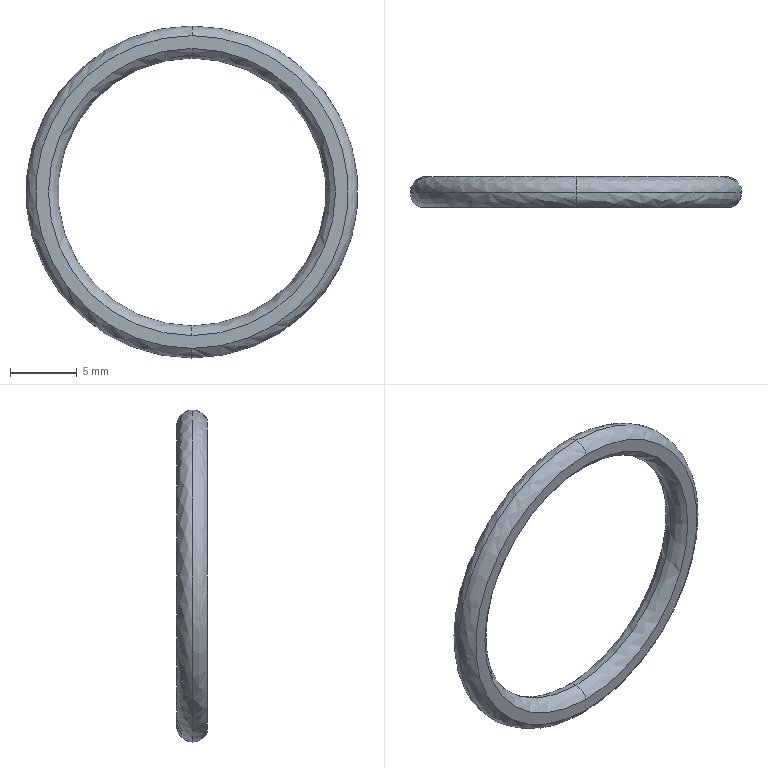Part | STEP file | PN_0034_default | 1 solid | 7 faces | box 24.8 x 2.3 x 24.8 mm | volume 313.815 mm3 | spline 6 | plane 1
STEP:
#1=CARTESIAN_POINT('',(0.,0.,0.));
#2=DIRECTION('',(0.,0.,1.));
#3=DIRECTION('',(1.,0.,0.));
#4=AXIS2_PLACEMENT_3D('',#1,#2,#3);
#5=CARTESIAN_POINT('',(0.,0.,10.));
#6=VERTEX_POINT('',#5);
#7=CARTESIAN_POINT('',(0.,0.,-10.));
#8=VERTEX_POINT('',#7);
#9=CARTESIAN_POINT('',(0.,0.,0.));
#10=DIRECTION('',(0.,-1.,0.));
#11=DIRECTION('',(0.,0.,-1.));
#12=AXIS2_PLACEMENT_3D('',#9,#10,#11);
#13=CIRCLE('',#12,10.);
#14=CARTESIAN_POINT('',(0.,0.,10.));
#15=CARTESIAN_POINT('',(-20.,0.,10.));
#16=CARTESIAN_POINT('',(-20.,0.,-10.));
#17=CARTESIAN_POINT('',(0.,0.,-10.));
#18=CARTESIAN_POINT('',(0.,-0.4919,10.));
#19=CARTESIAN_POINT('',(-20.,-0.4919,10.));
#20=CARTESIAN_POINT('',(-20.,-0.4919,-10.));
#21=CARTESIAN_POINT('',(0.,-0.4919,-10.));
#22=CARTESIAN_POINT('',(0.,-0.9034,10.27));
#23=CARTESIAN_POINT('',(-20.539,-0.9034,10.27));
#24=CARTESIAN_POINT('',(-20.539,-0.9034,-10.27));
#25=CARTESIAN_POINT('',(0.,-0.9034,-10.27));
#26=CARTESIAN_POINT('',(0.,-1.1,10.72));
#27=CARTESIAN_POINT('',(-21.441,-1.1,10.72));
#28=CARTESIAN_POINT('',(-21.441,-1.1,-10.72));
#29=CARTESIAN_POINT('',(0.,-1.1,-10.72));
#30=(BOUNDED_SURFACE()B_SPLINE_SURFACE(3,3,((#14,#15,#16,#17),(#18,#19,#20,#21),(#22,#23,#24,#25),(#26,#27,#28,#29)),.UNSPECIFIED.,.F.,.F.,.F.)B_SPLINE_SURFACE_WITH_KNOTS((4,4),(4,4),(0.,1.),(0.,1.),.PIECEWISE_BEZIER_KNOTS.)GEOMETRIC_REPRESENTATION_ITEM()RATIONAL_B_SPLINE_SURFACE(((1.,0.3333,0.3333,1.),(0.891,0.297,0.297,0.891),(0.891,0.297,0.297,0.891),(1.,0.3333,0.3333,1.)))REPRESENTATION_ITEM('')SURFACE());
#31=CARTESIAN_POINT('',(0.,0.));
#32=CARTESIAN_POINT('',(0.,0.02375));
#33=CARTESIAN_POINT('',(0.,0.06805));
#34=CARTESIAN_POINT('',(0.,0.1267));
#35=CARTESIAN_POINT('',(0.,0.1794));
#36=CARTESIAN_POINT('',(0.,0.2276));
#37=CARTESIAN_POINT('',(0.,0.2721));
#38=CARTESIAN_POINT('',(0.,0.3139));
#39=CARTESIAN_POINT('',(0.,0.3535));
#40=CARTESIAN_POINT('',(0.,0.3914));
#41=CARTESIAN_POINT('',(0.,0.4282));
#42=CARTESIAN_POINT('',(0.,0.4643));
#43=CARTESIAN_POINT('',(0.,0.5));
#44=CARTESIAN_POINT('',(0.,0.5357));
#45=CARTESIAN_POINT('',(0.,0.5718));
#46=CARTESIAN_POINT('',(0.,0.6086));
#47=CARTESIAN_POINT('',(0.,0.6465));
#48=CARTESIAN_POINT('',(0.,0.6861));
#49=CARTESIAN_POINT('',(0.,0.7279));
#50=CARTESIAN_POINT('',(0.,0.7724));
#51=CARTESIAN_POINT('',(0.,0.8206));
#52=CARTESIAN_POINT('',(0.,0.8733));
#53=CARTESIAN_POINT('',(0.,0.9319));
#54=CARTESIAN_POINT('',(0.,0.9763));
#55=CARTESIAN_POINT('',(0.,1.));
#56=B_SPLINE_CURVE_WITH_KNOTS('',3,(#31,#32,#33,#34,#35,#36,#37,#38,#39,#40,#41,#42,#43,#44,#45,#46,#47,#48,#49,#50,#51,#52,#53,#54,#55),.UNSPECIFIED.,.F.,.F.,(4,1,1,1,1,1,1,1,1,1,1,1,1,1,1,1,1,1,1,1,1,1,4),(3.142,3.284,3.427,3.57,3.713,3.856,3.998,4.141,4.284,4.427,4.57,4.712,4.855,4.998,5.141,5.284,5.426,5.569,5.712,5.855,5.998,6.14,6.283),.QUASI_UNIFORM_KNOTS.);
#57=(GEOMETRIC_REPRESENTATION_CONTEXT(2)PARAMETRIC_REPRESENTATION_CONTEXT()REPRESENTATION_CONTEXT('',''));
#58=DEFINITIONAL_REPRESENTATION('',(#56),#57);
#59=PCURVE('',#30,#58);
#60=CARTESIAN_POINT('',(0.,0.,12.4));
#61=CARTESIAN_POINT('',(-24.8,0.,12.4));
#62=CARTESIAN_POINT('',(-24.8,0.,-12.4));
#63=CARTESIAN_POINT('',(0.,0.,-12.4));
#64=CARTESIAN_POINT('',(0.,2.4,12.4));
#65=CARTESIAN_POINT('',(-24.8,2.4,12.4));
#66=CARTESIAN_POINT('',(-24.8,2.4,-12.4));
#67=CARTESIAN_POINT('',(0.,2.4,-12.4));
#68=CARTESIAN_POINT('',(0.,2.4,10.));
#69=CARTESIAN_POINT('',(-20.,2.4,10.));
#70=CARTESIAN_POINT('',(-20.,2.4,-10.));
#71=CARTESIAN_POINT('',(0.,2.4,-10.));
#72=CARTESIAN_POINT('',(0.,0.,10.));
#73=CARTESIAN_POINT('',(-20.,0.,10.));
#74=CARTESIAN_POINT('',(-20.,0.,-10.));
#75=CARTESIAN_POINT('',(0.,0.,-10.));
#76=(BOUNDED_SURFACE()B_SPLINE_SURFACE(3,3,((#60,#61,#62,#63),(#64,#65,#66,#67),(#68,#69,#70,#71),(#72,#73,#74,#75)),.UNSPECIFIED.,.F.,.F.,.F.)B_SPLINE_SURFACE_WITH_KNOTS((4,4),(4,4),(0.,1.),(0.,1.),.PIECEWISE_BEZIER_KNOTS.)GEOMETRIC_REPRESENTATION_ITEM()RATIONAL_B_SPLINE_SURFACE(((1.,0.3333,0.3333,1.),(0.3333,0.1111,0.1111,0.3333),(0.3333,0.1111,0.1111,0.3333),(1.,0.3333,0.3333,1.)))REPRESENTATION_ITEM('')SURFACE());
#77=CARTESIAN_POINT('',(1.,0.));
#78=CARTESIAN_POINT('',(1.,0.02375));
#79=CARTESIAN_POINT('',(1.,0.06805));
#80=CARTESIAN_POINT('',(1.,0.1267));
#81=CARTESIAN_POINT('',(1.,0.1794));
#82=CARTESIAN_POINT('',(1.,0.2276));
#83=CARTESIAN_POINT('',(1.,0.2721));
#84=CARTESIAN_POINT('',(1.,0.3139));
#85=CARTESIAN_POINT('',(1.,0.3535));
#86=CARTESIAN_POINT('',(1.,0.3914));
#87=CARTESIAN_POINT('',(1.,0.4282));
#88=CARTESIAN_POINT('',(1.,0.4643));
#89=CARTESIAN_POINT('',(1.,0.5));
#90=CARTESIAN_POINT('',(1.,0.5357));
#91=CARTESIAN_POINT('',(1.,0.5718));
#92=CARTESIAN_POINT('',(1.,0.6086));
#93=CARTESIAN_POINT('',(1.,0.6465));
#94=CARTESIAN_POINT('',(1.,0.6861));
#95=CARTESIAN_POINT('',(1.,0.7279));
#96=CARTESIAN_POINT('',(1.,0.7724));
#97=CARTESIAN_POINT('',(1.,0.8206));
#98=CARTESIAN_POINT('',(1.,0.8733));
#99=CARTESIAN_POINT('',(1.,0.9319));
#100=CARTESIAN_POINT('',(1.,0.9763));
#101=CARTESIAN_POINT('',(1.,1.));
#102=B_SPLINE_CURVE_WITH_KNOTS('',3,(#77,#78,#79,#80,#81,#82,#83,#84,#85,#86,#87,#88,#89,#90,#91,#92,#93,#94,#95,#96,#97,#98,#99,#100,#101),.UNSPECIFIED.,.F.,.F.,(4,1,1,1,1,1,1,1,1,1,1,1,1,1,1,1,1,1,1,1,1,1,4),(3.142,3.284,3.427,3.57,3.713,3.856,3.998,4.141,4.284,4.427,4.57,4.712,4.855,4.998,5.141,5.284,5.426,5.569,5.712,5.855,5.998,6.14,6.283),.QUASI_UNIFORM_KNOTS.);
#103=(GEOMETRIC_REPRESENTATION_CONTEXT(2)PARAMETRIC_REPRESENTATION_CONTEXT()REPRESENTATION_CONTEXT('',''));
#104=DEFINITIONAL_REPRESENTATION('',(#102),#103);
#105=PCURVE('',#76,#104);
#106=SURFACE_CURVE('',#13,(#59,#105),.PCURVE_S1.);
#107=EDGE_CURVE('',#6,#8,#106,.T.);
#108=ORIENTED_EDGE('',*,*,#107,.F.);
#109=CARTESIAN_POINT('',(0.,-1.1,10.72));
#110=VERTEX_POINT('',#109);
#111=CARTESIAN_POINT('',(0.,0.,11.2));
#112=DIRECTION('',(-1.,0.,0.));
#113=DIRECTION('',(0.,0.,1.));
#114=AXIS2_PLACEMENT_3D('',#111,#112,#113);
#115=CIRCLE('',#114,1.2);
#116=CARTESIAN_POINT('',(0.,0.));
#117=CARTESIAN_POINT('',(0.01603,0.));
#118=CARTESIAN_POINT('',(0.04785,0.));
#119=CARTESIAN_POINT('',(0.09491,0.));
#120=CARTESIAN_POINT('',(0.1414,0.));
#121=CARTESIAN_POINT('',(0.1873,0.));
#122=CARTESIAN_POINT('',(0.2328,0.));
#123=CARTESIAN_POINT('',(0.2779,0.));
#124=CARTESIAN_POINT('',(0.3227,0.));
#125=CARTESIAN_POINT('',(0.3672,0.));
#126=CARTESIAN_POINT('',(0.4116,0.));
#127=CARTESIAN_POINT('',(0.4558,0.));
#128=CARTESIAN_POINT('',(0.5,0.));
#129=CARTESIAN_POINT('',(0.5442,0.));
#130=CARTESIAN_POINT('',(0.5884,0.));
#131=CARTESIAN_POINT('',(0.6328,0.));
#132=CARTESIAN_POINT('',(0.6773,0.));
#133=CARTESIAN_POINT('',(0.7221,0.));
#134=CARTESIAN_POINT('',(0.7672,0.));
#135=CARTESIAN_POINT('',(0.8127,0.));
#136=CARTESIAN_POINT('',(0.8586,0.));
#137=CARTESIAN_POINT('',(0.9051,0.));
#138=CARTESIAN_POINT('',(0.9521,0.));
#139=CARTESIAN_POINT('',(0.984,0.));
#140=CARTESIAN_POINT('',(1.,0.));
#141=B_SPLINE_CURVE_WITH_KNOTS('',3,(#116,#117,#118,#119,#120,#121,#122,#123,#124,#125,#126,#127,#128,#129,#130,#131,#132,#133,#134,#135,#136,#137,#138,#139,#140),.UNSPECIFIED.,.F.,.F.,(4,1,1,1,1,1,1,1,1,1,1,1,1,1,1,1,1,1,1,1,1,1,4),(3.142,3.194,3.247,3.3,3.352,3.405,3.458,3.511,3.563,3.616,3.669,3.721,3.774,3.827,3.88,3.932,3.985,4.038,4.09,4.143,4.196,4.249,4.301),.QUASI_UNIFORM_KNOTS.);
#142=(GEOMETRIC_REPRESENTATION_CONTEXT(2)PARAMETRIC_REPRESENTATION_CONTEXT()REPRESENTATION_CONTEXT('',''));
#143=DEFINITIONAL_REPRESENTATION('',(#141),#142);
#144=PCURVE('',#30,#143);
#145=CARTESIAN_POINT('',(0.,0.,-10.));
#146=CARTESIAN_POINT('',(20.,0.,-10.));
#147=CARTESIAN_POINT('',(20.,0.,10.));
#148=CARTESIAN_POINT('',(0.,0.,10.));
#149=CARTESIAN_POINT('',(0.,-0.4919,-10.));
#150=CARTESIAN_POINT('',(20.,-0.4919,-10.));
#151=CARTESIAN_POINT('',(20.,-0.4919,10.));
#152=CARTESIAN_POINT('',(0.,-0.4919,10.));
#153=CARTESIAN_POINT('',(0.,-0.9034,-10.27));
#154=CARTESIAN_POINT('',(20.539,-0.9034,-10.27));
#155=CARTESIAN_POINT('',(20.539,-0.9034,10.27));
#156=CARTESIAN_POINT('',(0.,-0.9034,10.27));
#157=CARTESIAN_POINT('',(0.,-1.1,-10.72));
#158=CARTESIAN_POINT('',(21.441,-1.1,-10.72));
#159=CARTESIAN_POINT('',(21.441,-1.1,10.72));
#160=CARTESIAN_POINT('',(0.,-1.1,10.72));
#161=(BOUNDED_SURFACE()B_SPLINE_SURFACE(3,3,((#145,#146,#147,#148),(#149,#150,#151,#152),(#153,#154,#155,#156),(#157,#158,#159,#160)),.UNSPECIFIED.,.F.,.F.,.F.)B_SPLINE_SURFACE_WITH_KNOTS((4,4),(4,4),(0.,1.),(0.,1.),.PIECEWISE_BEZIER_KNOTS.)GEOMETRIC_REPRESENTATION_ITEM()RATIONAL_B_SPLINE_SURFACE(((1.,0.3333,0.3333,1.),(0.891,0.297,0.297,0.891),(0.891,0.297,0.297,0.891),(1.,0.3333,0.3333,1.)))REPRESENTATION_ITEM('')SURFACE());
#162=CARTESIAN_POINT('',(0.,1.));
#163=CARTESIAN_POINT('',(0.01603,1.));
#164=CARTESIAN_POINT('',(0.04785,1.));
#165=CARTESIAN_POINT('',(0.09491,1.));
#166=CARTESIAN_POINT('',(0.1414,1.));
#167=CARTESIAN_POINT('',(0.1873,1.));
#168=CARTESIAN_POINT('',(0.2328,1.));
#169=CARTESIAN_POINT('',(0.2779,1.));
#170=CARTESIAN_POINT('',(0.3227,1.));
#171=CARTESIAN_POINT('',(0.3672,1.));
#172=CARTESIAN_POINT('',(0.4116,1.));
#173=CARTESIAN_POINT('',(0.4558,1.));
#174=CARTESIAN_POINT('',(0.5,1.));
#175=CARTESIAN_POINT('',(0.5442,1.));
#176=CARTESIAN_POINT('',(0.5884,1.));
#177=CARTESIAN_POINT('',(0.6328,1.));
#178=CARTESIAN_POINT('',(0.6773,1.));
#179=CARTESIAN_POINT('',(0.7221,1.));
#180=CARTESIAN_POINT('',(0.7672,1.));
#181=CARTESIAN_POINT('',(0.8127,1.));
#182=CARTESIAN_POINT('',(0.8586,1.));
#183=CARTESIAN_POINT('',(0.9051,1.));
#184=CARTESIAN_POINT('',(0.9521,1.));
#185=CARTESIAN_POINT('',(0.984,1.));
#186=CARTESIAN_POINT('',(1.,1.));
#187=B_SPLINE_CURVE_WITH_KNOTS('',3,(#162,#163,#164,#165,#166,#167,#168,#169,#170,#171,#172,#173,#174,#175,#176,#177,#178,#179,#180,#181,#182,#183,#184,#185,#186),.UNSPECIFIED.,.F.,.F.,(4,1,1,1,1,1,1,1,1,1,1,1,1,1,1,1,1,1,1,1,1,1,4),(3.142,3.194,3.247,3.3,3.352,3.405,3.458,3.511,3.563,3.616,3.669,3.721,3.774,3.827,3.88,3.932,3.985,4.038,4.09,4.143,4.196,4.249,4.301),.QUASI_UNIFORM_KNOTS.);
#188=(GEOMETRIC_REPRESENTATION_CONTEXT(2)PARAMETRIC_REPRESENTATION_CONTEXT()REPRESENTATION_CONTEXT('',''));
#189=DEFINITIONAL_REPRESENTATION('',(#187),#188);
#190=PCURVE('',#161,#189);
#191=SURFACE_CURVE('',#115,(#144,#190),.PCURVE_S1.);
#192=EDGE_CURVE('',#6,#110,#191,.T.);
#193=ORIENTED_EDGE('',*,*,#192,.T.);
#194=CARTESIAN_POINT('',(0.,-1.1,-10.72));
#195=VERTEX_POINT('',#194);
#196=CARTESIAN_POINT('',(0.,-1.1,0.));
#197=DIRECTION('',(0.,-1.,0.));
#198=DIRECTION('',(0.,0.,-1.));
#199=AXIS2_PLACEMENT_3D('',#196,#197,#198);
#200=CIRCLE('',#199,10.72);
#201=CARTESIAN_POINT('',(1.,0.));
#202=CARTESIAN_POINT('',(1.,0.02375));
#203=CARTESIAN_POINT('',(1.,0.06805));
#204=CARTESIAN_POINT('',(1.,0.1267));
#205=CARTESIAN_POINT('',(1.,0.1794));
#206=CARTESIAN_POINT('',(1.,0.2276));
#207=CARTESIAN_POINT('',(1.,0.2721));
#208=CARTESIAN_POINT('',(1.,0.3139));
#209=CARTESIAN_POINT('',(1.,0.3535));
#210=CARTESIAN_POINT('',(1.,0.3914));
#211=CARTESIAN_POINT('',(1.,0.4282));
#212=CARTESIAN_POINT('',(1.,0.4643));
#213=CARTESIAN_POINT('',(1.,0.5));
#214=CARTESIAN_POINT('',(1.,0.5357));
#215=CARTESIAN_POINT('',(1.,0.5718));
#216=CARTESIAN_POINT('',(1.,0.6086));
#217=CARTESIAN_POINT('',(1.,0.6465));
#218=CARTESIAN_POINT('',(1.,0.6861));
#219=CARTESIAN_POINT('',(1.,0.7279));
#220=CARTESIAN_POINT('',(1.,0.7724));
#221=CARTESIAN_POINT('',(1.,0.8206));
#222=CARTESIAN_POINT('',(1.,0.8733));
#223=CARTESIAN_POINT('',(1.,0.9319));
#224=CARTESIAN_POINT('',(1.,0.9763));
#225=CARTESIAN_POINT('',(1.,1.));
#226=B_SPLINE_CURVE_WITH_KNOTS('',3,(#201,#202,#203,#204,#205,#206,#207,#208,#209,#210,#211,#212,#213,#214,#215,#216,#217,#218,#219,#220,#221,#222,#223,#224,#225),.UNSPECIFIED.,.F.,.F.,(4,1,1,1,1,1,1,1,1,1,1,1,1,1,1,1,1,1,1,1,1,1,4),(3.142,3.284,3.427,3.57,3.713,3.856,3.998,4.141,4.284,4.427,4.57,4.712,4.855,4.998,5.141,5.284,5.426,5.569,5.712,5.855,5.998,6.14,6.283),.QUASI_UNIFORM_KNOTS.);
#227=(GEOMETRIC_REPRESENTATION_CONTEXT(2)PARAMETRIC_REPRESENTATION_CONTEXT()REPRESENTATION_CONTEXT('',''));
#228=DEFINITIONAL_REPRESENTATION('',(#226),#227);
#229=PCURVE('',#30,#228);
#230=CARTESIAN_POINT('',(11.2,-1.1,0.));
#231=DIRECTION('',(0.,-1.,0.));
#232=DIRECTION('',(0.,0.,-1.));
#233=AXIS2_PLACEMENT_3D('',#230,#231,#232);
#234=PLANE('',#233);
#235=CARTESIAN_POINT('',(0.,-11.2));
#236=DIRECTION('',(1.,0.));
#237=AXIS2_PLACEMENT_2D('',#235,#236);
#238=CIRCLE('',#237,10.72);
#239=(GEOMETRIC_REPRESENTATION_CONTEXT(2)PARAMETRIC_REPRESENTATION_CONTEXT()REPRESENTATION_CONTEXT('',''));
#240=DEFINITIONAL_REPRESENTATION('',(#238),#239);
#241=PCURVE('',#234,#240);
#242=SURFACE_CURVE('',#200,(#229,#241),.PCURVE_S1.);
#243=EDGE_CURVE('',#110,#195,#242,.T.);
#244=ORIENTED_EDGE('',*,*,#243,.T.);
#245=CARTESIAN_POINT('',(0.,0.,-11.2));
#246=DIRECTION('',(1.,0.,0.));
#247=DIRECTION('',(0.,0.,-1.));
#248=AXIS2_PLACEMENT_3D('',#245,#246,#247);
#249=CIRCLE('',#248,1.2);
#250=CARTESIAN_POINT('',(0.,1.));
#251=CARTESIAN_POINT('',(0.01603,1.));
#252=CARTESIAN_POINT('',(0.04785,1.));
#253=CARTESIAN_POINT('',(0.09491,1.));
#254=CARTESIAN_POINT('',(0.1414,1.));
#255=CARTESIAN_POINT('',(0.1873,1.));
#256=CARTESIAN_POINT('',(0.2328,1.));
#257=CARTESIAN_POINT('',(0.2779,1.));
#258=CARTESIAN_POINT('',(0.3227,1.));
#259=CARTESIAN_POINT('',(0.3672,1.));
#260=CARTESIAN_POINT('',(0.4116,1.));
#261=CARTESIAN_POINT('',(0.4558,1.));
#262=CARTESIAN_POINT('',(0.5,1.));
#263=CARTESIAN_POINT('',(0.5442,1.));
#264=CARTESIAN_POINT('',(0.5884,1.));
#265=CARTESIAN_POINT('',(0.6328,1.));
#266=CARTESIAN_POINT('',(0.6773,1.));
#267=CARTESIAN_POINT('',(0.7221,1.));
#268=CARTESIAN_POINT('',(0.7672,1.));
#269=CARTESIAN_POINT('',(0.8127,1.));
#270=CARTESIAN_POINT('',(0.8586,1.));
#271=CARTESIAN_POINT('',(0.9051,1.));
#272=CARTESIAN_POINT('',(0.9521,1.));
#273=CARTESIAN_POINT('',(0.984,1.));
#274=CARTESIAN_POINT('',(1.,1.));
#275=B_SPLINE_CURVE_WITH_KNOTS('',3,(#250,#251,#252,#253,#254,#255,#256,#257,#258,#259,#260,#261,#262,#263,#264,#265,#266,#267,#268,#269,#270,#271,#272,#273,#274),.UNSPECIFIED.,.F.,.F.,(4,1,1,1,1,1,1,1,1,1,1,1,1,1,1,1,1,1,1,1,1,1,4),(3.142,3.194,3.247,3.3,3.352,3.405,3.458,3.511,3.563,3.616,3.669,3.721,3.774,3.827,3.88,3.932,3.985,4.038,4.09,4.143,4.196,4.249,4.301),.QUASI_UNIFORM_KNOTS.);
#276=(GEOMETRIC_REPRESENTATION_CONTEXT(2)PARAMETRIC_REPRESENTATION_CONTEXT()REPRESENTATION_CONTEXT('',''));
#277=DEFINITIONAL_REPRESENTATION('',(#275),#276);
#278=PCURVE('',#30,#277);
#279=CARTESIAN_POINT('',(0.,0.));
#280=CARTESIAN_POINT('',(0.01603,0.));
#281=CARTESIAN_POINT('',(0.04785,0.));
#282=CARTESIAN_POINT('',(0.09491,0.));
#283=CARTESIAN_POINT('',(0.1414,0.));
#284=CARTESIAN_POINT('',(0.1873,0.));
#285=CARTESIAN_POINT('',(0.2328,0.));
#286=CARTESIAN_POINT('',(0.2779,0.));
#287=CARTESIAN_POINT('',(0.3227,0.));
#288=CARTESIAN_POINT('',(0.3672,0.));
#289=CARTESIAN_POINT('',(0.4116,0.));
#290=CARTESIAN_POINT('',(0.4558,0.));
#291=CARTESIAN_POINT('',(0.5,0.));
#292=CARTESIAN_POINT('',(0.5442,0.));
#293=CARTESIAN_POINT('',(0.5884,0.));
#294=CARTESIAN_POINT('',(0.6328,0.));
#295=CARTESIAN_POINT('',(0.6773,0.));
#296=CARTESIAN_POINT('',(0.7221,0.));
#297=CARTESIAN_POINT('',(0.7672,0.));
#298=CARTESIAN_POINT('',(0.8127,0.));
#299=CARTESIAN_POINT('',(0.8586,0.));
#300=CARTESIAN_POINT('',(0.9051,0.));
#301=CARTESIAN_POINT('',(0.9521,0.));
#302=CARTESIAN_POINT('',(0.984,0.));
#303=CARTESIAN_POINT('',(1.,0.));
#304=B_SPLINE_CURVE_WITH_KNOTS('',3,(#279,#280,#281,#282,#283,#284,#285,#286,#287,#288,#289,#290,#291,#292,#293,#294,#295,#296,#297,#298,#299,#300,#301,#302,#303),.UNSPECIFIED.,.F.,.F.,(4,1,1,1,1,1,1,1,1,1,1,1,1,1,1,1,1,1,1,1,1,1,4),(3.142,3.194,3.247,3.3,3.352,3.405,3.458,3.511,3.563,3.616,3.669,3.721,3.774,3.827,3.88,3.932,3.985,4.038,4.09,4.143,4.196,4.249,4.301),.QUASI_UNIFORM_KNOTS.);
#305=(GEOMETRIC_REPRESENTATION_CONTEXT(2)PARAMETRIC_REPRESENTATION_CONTEXT()REPRESENTATION_CONTEXT('',''));
#306=DEFINITIONAL_REPRESENTATION('',(#304),#305);
#307=PCURVE('',#161,#306);
#308=SURFACE_CURVE('',#249,(#278,#307),.PCURVE_S1.);
#309=EDGE_CURVE('',#8,#195,#308,.T.);
#310=ORIENTED_EDGE('',*,*,#309,.F.);
#311=EDGE_LOOP('',(#108,#193,#244,#310));
#312=FACE_BOUND('',#311,.T.);
#313=ADVANCED_FACE('',(#312),#30,.T.);
#314=CARTESIAN_POINT('',(0.,-1.1,-11.68));
#315=VERTEX_POINT('',#314);
#316=CARTESIAN_POINT('',(0.,-1.1,11.68));
#317=VERTEX_POINT('',#316);
#318=CARTESIAN_POINT('',(0.,-1.1,0.));
#319=DIRECTION('',(0.,1.,0.));
#320=DIRECTION('',(0.,0.,-1.));
#321=AXIS2_PLACEMENT_3D('',#318,#319,#320);
#322=CIRCLE('',#321,11.68);
#323=CARTESIAN_POINT('',(0.,-1.1,11.68));
#324=CARTESIAN_POINT('',(-23.359,-1.1,11.68));
#325=CARTESIAN_POINT('',(-23.359,-1.1,-11.68));
#326=CARTESIAN_POINT('',(0.,-1.1,-11.68));
#327=CARTESIAN_POINT('',(0.,-0.9034,12.13));
#328=CARTESIAN_POINT('',(-24.261,-0.9034,12.13));
#329=CARTESIAN_POINT('',(-24.261,-0.9034,-12.13));
#330=CARTESIAN_POINT('',(0.,-0.9034,-12.13));
#331=CARTESIAN_POINT('',(0.,-0.4919,12.4));
#332=CARTESIAN_POINT('',(-24.8,-0.4919,12.4));
#333=CARTESIAN_POINT('',(-24.8,-0.4919,-12.4));
#334=CARTESIAN_POINT('',(0.,-0.4919,-12.4));
#335=CARTESIAN_POINT('',(0.,0.,12.4));
#336=CARTESIAN_POINT('',(-24.8,0.,12.4));
#337=CARTESIAN_POINT('',(-24.8,0.,-12.4));
#338=CARTESIAN_POINT('',(0.,0.,-12.4));
#339=(BOUNDED_SURFACE()B_SPLINE_SURFACE(3,3,((#323,#324,#325,#326),(#327,#328,#329,#330),(#331,#332,#333,#334),(#335,#336,#337,#338)),.UNSPECIFIED.,.F.,.F.,.F.)B_SPLINE_SURFACE_WITH_KNOTS((4,4),(4,4),(0.,1.),(0.,1.),.PIECEWISE_BEZIER_KNOTS.)GEOMETRIC_REPRESENTATION_ITEM()RATIONAL_B_SPLINE_SURFACE(((1.,0.3333,0.3333,1.),(0.891,0.297,0.297,0.891),(0.891,0.297,0.297,0.891),(1.,0.3333,0.3333,1.)))REPRESENTATION_ITEM('')SURFACE());
#340=CARTESIAN_POINT('',(0.,1.));
#341=CARTESIAN_POINT('',(0.,0.9763));
#342=CARTESIAN_POINT('',(0.,0.9319));
#343=CARTESIAN_POINT('',(0.,0.8733));
#344=CARTESIAN_POINT('',(0.,0.8206));
#345=CARTESIAN_POINT('',(0.,0.7724));
#346=CARTESIAN_POINT('',(0.,0.7279));
#347=CARTESIAN_POINT('',(0.,0.6861));
#348=CARTESIAN_POINT('',(0.,0.6465));
#349=CARTESIAN_POINT('',(0.,0.6086));
#350=CARTESIAN_POINT('',(0.,0.5718));
#351=CARTESIAN_POINT('',(0.,0.5357));
#352=CARTESIAN_POINT('',(0.,0.5));
#353=CARTESIAN_POINT('',(0.,0.4643));
#354=CARTESIAN_POINT('',(0.,0.4282));
#355=CARTESIAN_POINT('',(0.,0.3914));
#356=CARTESIAN_POINT('',(0.,0.3535));
#357=CARTESIAN_POINT('',(0.,0.3139));
#358=CARTESIAN_POINT('',(0.,0.2721));
#359=CARTESIAN_POINT('',(0.,0.2276));
#360=CARTESIAN_POINT('',(0.,0.1794));
#361=CARTESIAN_POINT('',(0.,0.1267));
#362=CARTESIAN_POINT('',(0.,0.06805));
#363=CARTESIAN_POINT('',(0.,0.02375));
#364=CARTESIAN_POINT('',(0.,0.));
#365=B_SPLINE_CURVE_WITH_KNOTS('',3,(#340,#341,#342,#343,#344,#345,#346,#347,#348,#349,#350,#351,#352,#353,#354,#355,#356,#357,#358,#359,#360,#361,#362,#363,#364),.UNSPECIFIED.,.F.,.F.,(4,1,1,1,1,1,1,1,1,1,1,1,1,1,1,1,1,1,1,1,1,1,4),(0.,0.1428,0.2856,0.4284,0.5712,0.714,0.8568,0.9996,1.142,1.285,1.428,1.571,1.714,1.856,1.999,2.142,2.285,2.428,2.57,2.713,2.856,2.999,3.142),.QUASI_UNIFORM_KNOTS.);
#366=(GEOMETRIC_REPRESENTATION_CONTEXT(2)PARAMETRIC_REPRESENTATION_CONTEXT()REPRESENTATION_CONTEXT('',''));
#367=DEFINITIONAL_REPRESENTATION('',(#365),#366);
#368=PCURVE('',#339,#367);
#369=CARTESIAN_POINT('',(11.68,-11.2));
#370=CARTESIAN_POINT('',(11.68,-31.43));
#371=CARTESIAN_POINT('',(-5.84,-21.315));
#372=CARTESIAN_POINT('',(-23.359,-11.2));
#373=CARTESIAN_POINT('',(-5.84,-1.085));
#374=CARTESIAN_POINT('',(11.68,9.03));
#375=CARTESIAN_POINT('',(11.68,-11.2));
#376=(BOUNDED_CURVE()B_SPLINE_CURVE(2,(#369,#370,#371,#372,#373,#374,#375),.UNSPECIFIED.,.T.,.F.)B_SPLINE_CURVE_WITH_KNOTS((1,2,2,2,2,1),(-2.094,0.,2.094,4.189,6.283,8.378),.UNSPECIFIED.)CURVE()GEOMETRIC_REPRESENTATION_ITEM()RATIONAL_B_SPLINE_CURVE((1.,0.5,1.,0.5,1.,0.5,1.))REPRESENTATION_ITEM(''));
#377=(GEOMETRIC_REPRESENTATION_CONTEXT(2)PARAMETRIC_REPRESENTATION_CONTEXT()REPRESENTATION_CONTEXT('',''));
#378=DEFINITIONAL_REPRESENTATION('',(#376),#377);
#379=PCURVE('',#234,#378);
#380=SURFACE_CURVE('',#322,(#368,#379),.PCURVE_S1.);
#381=EDGE_CURVE('',#315,#317,#380,.T.);
#382=ORIENTED_EDGE('',*,*,#381,.T.);
#383=CARTESIAN_POINT('',(0.,0.,12.4));
#384=VERTEX_POINT('',#383);
#385=CARTESIAN_POINT('',(0.,0.,11.2));
#386=DIRECTION('',(-1.,0.,0.));
#387=DIRECTION('',(0.,0.,1.));
#388=AXIS2_PLACEMENT_3D('',#385,#386,#387);
#389=CIRCLE('',#388,1.2);
#390=CARTESIAN_POINT('',(0.,0.));
#391=CARTESIAN_POINT('',(0.01603,0.));
#392=CARTESIAN_POINT('',(0.04785,0.));
#393=CARTESIAN_POINT('',(0.09491,0.));
#394=CARTESIAN_POINT('',(0.1414,0.));
#395=CARTESIAN_POINT('',(0.1873,0.));
#396=CARTESIAN_POINT('',(0.2328,0.));
#397=CARTESIAN_POINT('',(0.2779,0.));
#398=CARTESIAN_POINT('',(0.3227,0.));
#399=CARTESIAN_POINT('',(0.3672,0.));
#400=CARTESIAN_POINT('',(0.4116,0.));
#401=CARTESIAN_POINT('',(0.4558,0.));
#402=CARTESIAN_POINT('',(0.5,0.));
#403=CARTESIAN_POINT('',(0.5442,0.));
#404=CARTESIAN_POINT('',(0.5884,0.));
#405=CARTESIAN_POINT('',(0.6328,0.));
#406=CARTESIAN_POINT('',(0.6773,0.));
#407=CARTESIAN_POINT('',(0.7221,0.));
#408=CARTESIAN_POINT('',(0.7672,0.));
#409=CARTESIAN_POINT('',(0.8127,0.));
#410=CARTESIAN_POINT('',(0.8586,0.));
#411=CARTESIAN_POINT('',(0.9051,0.));
#412=CARTESIAN_POINT('',(0.9521,0.));
#413=CARTESIAN_POINT('',(0.984,0.));
#414=CARTESIAN_POINT('',(1.,0.));
#415=B_SPLINE_CURVE_WITH_KNOTS('',3,(#390,#391,#392,#393,#394,#395,#396,#397,#398,#399,#400,#401,#402,#403,#404,#405,#406,#407,#408,#409,#410,#411,#412,#413,#414),.UNSPECIFIED.,.F.,.F.,(4,1,1,1,1,1,1,1,1,1,1,1,1,1,1,1,1,1,1,1,1,1,4),(5.124,5.176,5.229,5.282,5.334,5.387,5.44,5.493,5.545,5.598,5.651,5.703,5.756,5.809,5.861,5.914,5.967,6.02,6.072,6.125,6.178,6.23,6.283),.QUASI_UNIFORM_KNOTS.);
#416=(GEOMETRIC_REPRESENTATION_CONTEXT(2)PARAMETRIC_REPRESENTATION_CONTEXT()REPRESENTATION_CONTEXT('',''));
#417=DEFINITIONAL_REPRESENTATION('',(#415),#416);
#418=PCURVE('',#339,#417);
#419=CARTESIAN_POINT('',(0.,-1.1,-11.68));
#420=CARTESIAN_POINT('',(23.359,-1.1,-11.68));
#421=CARTESIAN_POINT('',(23.359,-1.1,11.68));
#422=CARTESIAN_POINT('',(0.,-1.1,11.68));
#423=CARTESIAN_POINT('',(0.,-0.9034,-12.13));
#424=CARTESIAN_POINT('',(24.261,-0.9034,-12.13));
#425=CARTESIAN_POINT('',(24.261,-0.9034,12.13));
#426=CARTESIAN_POINT('',(0.,-0.9034,12.13));
#427=CARTESIAN_POINT('',(0.,-0.4919,-12.4));
#428=CARTESIAN_POINT('',(24.8,-0.4919,-12.4));
#429=CARTESIAN_POINT('',(24.8,-0.4919,12.4));
#430=CARTESIAN_POINT('',(0.,-0.4919,12.4));
#431=CARTESIAN_POINT('',(0.,0.,-12.4));
#432=CARTESIAN_POINT('',(24.8,0.,-12.4));
#433=CARTESIAN_POINT('',(24.8,0.,12.4));
#434=CARTESIAN_POINT('',(0.,0.,12.4));
#435=(BOUNDED_SURFACE()B_SPLINE_SURFACE(3,3,((#419,#420,#421,#422),(#423,#424,#425,#426),(#427,#428,#429,#430),(#431,#432,#433,#434)),.UNSPECIFIED.,.F.,.F.,.F.)B_SPLINE_SURFACE_WITH_KNOTS((4,4),(4,4),(0.,1.),(0.,1.),.PIECEWISE_BEZIER_KNOTS.)GEOMETRIC_REPRESENTATION_ITEM()RATIONAL_B_SPLINE_SURFACE(((1.,0.3333,0.3333,1.),(0.891,0.297,0.297,0.891),(0.891,0.297,0.297,0.891),(1.,0.3333,0.3333,1.)))REPRESENTATION_ITEM('')SURFACE());
#436=CARTESIAN_POINT('',(0.,1.));
#437=CARTESIAN_POINT('',(0.01603,1.));
#438=CARTESIAN_POINT('',(0.04785,1.));
#439=CARTESIAN_POINT('',(0.09491,1.));
#440=CARTESIAN_POINT('',(0.1414,1.));
#441=CARTESIAN_POINT('',(0.1873,1.));
#442=CARTESIAN_POINT('',(0.2328,1.));
#443=CARTESIAN_POINT('',(0.2779,1.));
#444=CARTESIAN_POINT('',(0.3227,1.));
#445=CARTESIAN_POINT('',(0.3672,1.));
#446=CARTESIAN_POINT('',(0.4116,1.));
#447=CARTESIAN_POINT('',(0.4558,1.));
#448=CARTESIAN_POINT('',(0.5,1.));
#449=CARTESIAN_POINT('',(0.5442,1.));
#450=CARTESIAN_POINT('',(0.5884,1.));
#451=CARTESIAN_POINT('',(0.6328,1.));
#452=CARTESIAN_POINT('',(0.6773,1.));
#453=CARTESIAN_POINT('',(0.7221,1.));
#454=CARTESIAN_POINT('',(0.7672,1.));
#455=CARTESIAN_POINT('',(0.8127,1.));
#456=CARTESIAN_POINT('',(0.8586,1.));
#457=CARTESIAN_POINT('',(0.9051,1.));
#458=CARTESIAN_POINT('',(0.9521,1.));
#459=CARTESIAN_POINT('',(0.984,1.));
#460=CARTESIAN_POINT('',(1.,1.));
#461=B_SPLINE_CURVE_WITH_KNOTS('',3,(#436,#437,#438,#439,#440,#441,#442,#443,#444,#445,#446,#447,#448,#449,#450,#451,#452,#453,#454,#455,#456,#457,#458,#459,#460),.UNSPECIFIED.,.F.,.F.,(4,1,1,1,1,1,1,1,1,1,1,1,1,1,1,1,1,1,1,1,1,1,4),(5.124,5.176,5.229,5.282,5.334,5.387,5.44,5.493,5.545,5.598,5.651,5.703,5.756,5.809,5.861,5.914,5.967,6.02,6.072,6.125,6.178,6.23,6.283),.QUASI_UNIFORM_KNOTS.);
#462=(GEOMETRIC_REPRESENTATION_CONTEXT(2)PARAMETRIC_REPRESENTATION_CONTEXT()REPRESENTATION_CONTEXT('',''));
#463=DEFINITIONAL_REPRESENTATION('',(#461),#462);
#464=PCURVE('',#435,#463);
#465=SURFACE_CURVE('',#389,(#418,#464),.PCURVE_S1.);
#466=EDGE_CURVE('',#317,#384,#465,.T.);
#467=ORIENTED_EDGE('',*,*,#466,.T.);
#468=CARTESIAN_POINT('',(0.,0.,-12.4));
#469=VERTEX_POINT('',#468);
#470=CARTESIAN_POINT('',(0.,0.,0.));
#471=DIRECTION('',(0.,-1.,0.));
#472=DIRECTION('',(0.,0.,-1.));
#473=AXIS2_PLACEMENT_3D('',#470,#471,#472);
#474=CIRCLE('',#473,12.4);
#475=CARTESIAN_POINT('',(1.,0.));
#476=CARTESIAN_POINT('',(1.,0.02375));
#477=CARTESIAN_POINT('',(1.,0.06805));
#478=CARTESIAN_POINT('',(1.,0.1267));
#479=CARTESIAN_POINT('',(1.,0.1794));
#480=CARTESIAN_POINT('',(1.,0.2276));
#481=CARTESIAN_POINT('',(1.,0.2721));
#482=CARTESIAN_POINT('',(1.,0.3139));
#483=CARTESIAN_POINT('',(1.,0.3535));
#484=CARTESIAN_POINT('',(1.,0.3914));
#485=CARTESIAN_POINT('',(1.,0.4282));
#486=CARTESIAN_POINT('',(1.,0.4643));
#487=CARTESIAN_POINT('',(1.,0.5));
#488=CARTESIAN_POINT('',(1.,0.5357));
#489=CARTESIAN_POINT('',(1.,0.5718));
#490=CARTESIAN_POINT('',(1.,0.6086));
#491=CARTESIAN_POINT('',(1.,0.6465));
#492=CARTESIAN_POINT('',(1.,0.6861));
#493=CARTESIAN_POINT('',(1.,0.7279));
#494=CARTESIAN_POINT('',(1.,0.7724));
#495=CARTESIAN_POINT('',(1.,0.8206));
#496=CARTESIAN_POINT('',(1.,0.8733));
#497=CARTESIAN_POINT('',(1.,0.9319));
#498=CARTESIAN_POINT('',(1.,0.9763));
#499=CARTESIAN_POINT('',(1.,1.));
#500=B_SPLINE_CURVE_WITH_KNOTS('',3,(#475,#476,#477,#478,#479,#480,#481,#482,#483,#484,#485,#486,#487,#488,#489,#490,#491,#492,#493,#494,#495,#496,#497,#498,#499),.UNSPECIFIED.,.F.,.F.,(4,1,1,1,1,1,1,1,1,1,1,1,1,1,1,1,1,1,1,1,1,1,4),(3.142,3.284,3.427,3.57,3.713,3.856,3.998,4.141,4.284,4.427,4.57,4.712,4.855,4.998,5.141,5.284,5.426,5.569,5.712,5.855,5.998,6.14,6.283),.QUASI_UNIFORM_KNOTS.);
#501=(GEOMETRIC_REPRESENTATION_CONTEXT(2)PARAMETRIC_REPRESENTATION_CONTEXT()REPRESENTATION_CONTEXT('',''));
#502=DEFINITIONAL_REPRESENTATION('',(#500),#501);
#503=PCURVE('',#339,#502);
#504=CARTESIAN_POINT('',(0.,0.));
#505=CARTESIAN_POINT('',(0.,0.02375));
#506=CARTESIAN_POINT('',(0.,0.06805));
#507=CARTESIAN_POINT('',(0.,0.1267));
#508=CARTESIAN_POINT('',(0.,0.1794));
#509=CARTESIAN_POINT('',(0.,0.2276));
#510=CARTESIAN_POINT('',(0.,0.2721));
#511=CARTESIAN_POINT('',(0.,0.3139));
#512=CARTESIAN_POINT('',(0.,0.3535));
#513=CARTESIAN_POINT('',(0.,0.3914));
#514=CARTESIAN_POINT('',(0.,0.4282));
#515=CARTESIAN_POINT('',(0.,0.4643));
#516=CARTESIAN_POINT('',(0.,0.5));
#517=CARTESIAN_POINT('',(0.,0.5357));
#518=CARTESIAN_POINT('',(0.,0.5718));
#519=CARTESIAN_POINT('',(0.,0.6086));
#520=CARTESIAN_POINT('',(0.,0.6465));
#521=CARTESIAN_POINT('',(0.,0.6861));
#522=CARTESIAN_POINT('',(0.,0.7279));
#523=CARTESIAN_POINT('',(0.,0.7724));
#524=CARTESIAN_POINT('',(0.,0.8206));
#525=CARTESIAN_POINT('',(0.,0.8733));
#526=CARTESIAN_POINT('',(0.,0.9319));
#527=CARTESIAN_POINT('',(0.,0.9763));
#528=CARTESIAN_POINT('',(0.,1.));
#529=B_SPLINE_CURVE_WITH_KNOTS('',3,(#504,#505,#506,#507,#508,#509,#510,#511,#512,#513,#514,#515,#516,#517,#518,#519,#520,#521,#522,#523,#524,#525,#526,#527,#528),.UNSPECIFIED.,.F.,.F.,(4,1,1,1,1,1,1,1,1,1,1,1,1,1,1,1,1,1,1,1,1,1,4),(3.142,3.284,3.427,3.57,3.713,3.856,3.998,4.141,4.284,4.427,4.57,4.712,4.855,4.998,5.141,5.284,5.426,5.569,5.712,5.855,5.998,6.14,6.283),.QUASI_UNIFORM_KNOTS.);
#530=(GEOMETRIC_REPRESENTATION_CONTEXT(2)PARAMETRIC_REPRESENTATION_CONTEXT()REPRESENTATION_CONTEXT('',''));
#531=DEFINITIONAL_REPRESENTATION('',(#529),#530);
#532=PCURVE('',#76,#531);
#533=SURFACE_CURVE('',#474,(#503,#532),.PCURVE_S1.);
#534=EDGE_CURVE('',#384,#469,#533,.T.);
#535=ORIENTED_EDGE('',*,*,#534,.T.);
#536=CARTESIAN_POINT('',(0.,0.,-11.2));
#537=DIRECTION('',(1.,0.,0.));
#538=DIRECTION('',(0.,0.,-1.));
#539=AXIS2_PLACEMENT_3D('',#536,#537,#538);
#540=CIRCLE('',#539,1.2);
#541=CARTESIAN_POINT('',(0.,1.));
#542=CARTESIAN_POINT('',(0.01603,1.));
#543=CARTESIAN_POINT('',(0.04785,1.));
#544=CARTESIAN_POINT('',(0.09491,1.));
#545=CARTESIAN_POINT('',(0.1414,1.));
#546=CARTESIAN_POINT('',(0.1873,1.));
#547=CARTESIAN_POINT('',(0.2328,1.));
#548=CARTESIAN_POINT('',(0.2779,1.));
#549=CARTESIAN_POINT('',(0.3227,1.));
#550=CARTESIAN_POINT('',(0.3672,1.));
#551=CARTESIAN_POINT('',(0.4116,1.));
#552=CARTESIAN_POINT('',(0.4558,1.));
#553=CARTESIAN_POINT('',(0.5,1.));
#554=CARTESIAN_POINT('',(0.5442,1.));
#555=CARTESIAN_POINT('',(0.5884,1.));
#556=CARTESIAN_POINT('',(0.6328,1.));
#557=CARTESIAN_POINT('',(0.6773,1.));
#558=CARTESIAN_POINT('',(0.7221,1.));
#559=CARTESIAN_POINT('',(0.7672,1.));
#560=CARTESIAN_POINT('',(0.8127,1.));
#561=CARTESIAN_POINT('',(0.8586,1.));
#562=CARTESIAN_POINT('',(0.9051,1.));
#563=CARTESIAN_POINT('',(0.9521,1.));
#564=CARTESIAN_POINT('',(0.984,1.));
#565=CARTESIAN_POINT('',(1.,1.));
#566=B_SPLINE_CURVE_WITH_KNOTS('',3,(#541,#542,#543,#544,#545,#546,#547,#548,#549,#550,#551,#552,#553,#554,#555,#556,#557,#558,#559,#560,#561,#562,#563,#564,#565),.UNSPECIFIED.,.F.,.F.,(4,1,1,1,1,1,1,1,1,1,1,1,1,1,1,1,1,1,1,1,1,1,4),(5.124,5.176,5.229,5.282,5.334,5.387,5.44,5.493,5.545,5.598,5.651,5.703,5.756,5.809,5.861,5.914,5.967,6.02,6.072,6.125,6.178,6.23,6.283),.QUASI_UNIFORM_KNOTS.);
#567=(GEOMETRIC_REPRESENTATION_CONTEXT(2)PARAMETRIC_REPRESENTATION_CONTEXT()REPRESENTATION_CONTEXT('',''));
#568=DEFINITIONAL_REPRESENTATION('',(#566),#567);
#569=PCURVE('',#339,#568);
#570=CARTESIAN_POINT('',(0.,0.));
#571=CARTESIAN_POINT('',(0.01603,0.));
#572=CARTESIAN_POINT('',(0.04785,0.));
#573=CARTESIAN_POINT('',(0.09491,0.));
#574=CARTESIAN_POINT('',(0.1414,0.));
#575=CARTESIAN_POINT('',(0.1873,0.));
#576=CARTESIAN_POINT('',(0.2328,0.));
#577=CARTESIAN_POINT('',(0.2779,0.));
#578=CARTESIAN_POINT('',(0.3227,0.));
#579=CARTESIAN_POINT('',(0.3672,0.));
#580=CARTESIAN_POINT('',(0.4116,0.));
#581=CARTESIAN_POINT('',(0.4558,0.));
#582=CARTESIAN_POINT('',(0.5,0.));
#583=CARTESIAN_POINT('',(0.5442,0.));
#584=CARTESIAN_POINT('',(0.5884,0.));
#585=CARTESIAN_POINT('',(0.6328,0.));
#586=CARTESIAN_POINT('',(0.6773,0.));
#587=CARTESIAN_POINT('',(0.7221,0.));
#588=CARTESIAN_POINT('',(0.7672,0.));
#589=CARTESIAN_POINT('',(0.8127,0.));
#590=CARTESIAN_POINT('',(0.8586,0.));
#591=CARTESIAN_POINT('',(0.9051,0.));
#592=CARTESIAN_POINT('',(0.9521,0.));
#593=CARTESIAN_POINT('',(0.984,0.));
#594=CARTESIAN_POINT('',(1.,0.));
#595=B_SPLINE_CURVE_WITH_KNOTS('',3,(#570,#571,#572,#573,#574,#575,#576,#577,#578,#579,#580,#581,#582,#583,#584,#585,#586,#587,#588,#589,#590,#591,#592,#593,#594),.UNSPECIFIED.,.F.,.F.,(4,1,1,1,1,1,1,1,1,1,1,1,1,1,1,1,1,1,1,1,1,1,4),(5.124,5.176,5.229,5.282,5.334,5.387,5.44,5.493,5.545,5.598,5.651,5.703,5.756,5.809,5.861,5.914,5.967,6.02,6.072,6.125,6.178,6.23,6.283),.QUASI_UNIFORM_KNOTS.);
#596=(GEOMETRIC_REPRESENTATION_CONTEXT(2)PARAMETRIC_REPRESENTATION_CONTEXT()REPRESENTATION_CONTEXT('',''));
#597=DEFINITIONAL_REPRESENTATION('',(#595),#596);
#598=PCURVE('',#435,#597);
#599=SURFACE_CURVE('',#540,(#569,#598),.PCURVE_S1.);
#600=EDGE_CURVE('',#315,#469,#599,.T.);
#601=ORIENTED_EDGE('',*,*,#600,.F.);
#602=EDGE_LOOP('',(#382,#467,#535,#601));
#603=FACE_BOUND('',#602,.T.);
#604=ADVANCED_FACE('',(#603),#339,.T.);
#605=ORIENTED_EDGE('',*,*,#534,.F.);
#606=CARTESIAN_POINT('',(0.,0.,11.2));
#607=DIRECTION('',(-1.,0.,0.));
#608=DIRECTION('',(0.,0.,1.));
#609=AXIS2_PLACEMENT_3D('',#606,#607,#608);
#610=CIRCLE('',#609,1.2);
#611=CARTESIAN_POINT('',(0.,0.));
#612=CARTESIAN_POINT('',(0.02375,0.));
#613=CARTESIAN_POINT('',(0.06805,0.));
#614=CARTESIAN_POINT('',(0.1267,0.));
#615=CARTESIAN_POINT('',(0.1794,0.));
#616=CARTESIAN_POINT('',(0.2276,0.));
#617=CARTESIAN_POINT('',(0.2721,0.));
#618=CARTESIAN_POINT('',(0.3139,0.));
#619=CARTESIAN_POINT('',(0.3535,0.));
#620=CARTESIAN_POINT('',(0.3914,0.));
#621=CARTESIAN_POINT('',(0.4282,0.));
#622=CARTESIAN_POINT('',(0.4643,0.));
#623=CARTESIAN_POINT('',(0.5,0.));
#624=CARTESIAN_POINT('',(0.5357,0.));
#625=CARTESIAN_POINT('',(0.5718,0.));
#626=CARTESIAN_POINT('',(0.6086,0.));
#627=CARTESIAN_POINT('',(0.6465,0.));
#628=CARTESIAN_POINT('',(0.6861,0.));
#629=CARTESIAN_POINT('',(0.7279,0.));
#630=CARTESIAN_POINT('',(0.7724,0.));
#631=CARTESIAN_POINT('',(0.8206,0.));
#632=CARTESIAN_POINT('',(0.8733,0.));
#633=CARTESIAN_POINT('',(0.9319,0.));
#634=CARTESIAN_POINT('',(0.9763,0.));
#635=CARTESIAN_POINT('',(1.,0.));
#636=B_SPLINE_CURVE_WITH_KNOTS('',3,(#611,#612,#613,#614,#615,#616,#617,#618,#619,#620,#621,#622,#623,#624,#625,#626,#627,#628,#629,#630,#631,#632,#633,#634,#635),.UNSPECIFIED.,.F.,.F.,(4,1,1,1,1,1,1,1,1,1,1,1,1,1,1,1,1,1,1,1,1,1,4),(0.,0.1428,0.2856,0.4284,0.5712,0.714,0.8568,0.9996,1.142,1.285,1.428,1.571,1.714,1.856,1.999,2.142,2.285,2.428,2.57,2.713,2.856,2.999,3.142),.QUASI_UNIFORM_KNOTS.);
#637=(GEOMETRIC_REPRESENTATION_CONTEXT(2)PARAMETRIC_REPRESENTATION_CONTEXT()REPRESENTATION_CONTEXT('',''));
#638=DEFINITIONAL_REPRESENTATION('',(#636),#637);
#639=PCURVE('',#76,#638);
#640=CARTESIAN_POINT('',(0.,0.,-12.4));
#641=CARTESIAN_POINT('',(24.8,0.,-12.4));
#642=CARTESIAN_POINT('',(24.8,0.,12.4));
#643=CARTESIAN_POINT('',(0.,0.,12.4));
#644=CARTESIAN_POINT('',(0.,2.4,-12.4));
#645=CARTESIAN_POINT('',(24.8,2.4,-12.4));
#646=CARTESIAN_POINT('',(24.8,2.4,12.4));
#647=CARTESIAN_POINT('',(0.,2.4,12.4));
#648=CARTESIAN_POINT('',(0.,2.4,-10.));
#649=CARTESIAN_POINT('',(20.,2.4,-10.));
#650=CARTESIAN_POINT('',(20.,2.4,10.));
#651=CARTESIAN_POINT('',(0.,2.4,10.));
#652=CARTESIAN_POINT('',(0.,0.,-10.));
#653=CARTESIAN_POINT('',(20.,0.,-10.));
#654=CARTESIAN_POINT('',(20.,0.,10.));
#655=CARTESIAN_POINT('',(0.,0.,10.));
#656=(BOUNDED_SURFACE()B_SPLINE_SURFACE(3,3,((#640,#641,#642,#643),(#644,#645,#646,#647),(#648,#649,#650,#651),(#652,#653,#654,#655)),.UNSPECIFIED.,.F.,.F.,.F.)B_SPLINE_SURFACE_WITH_KNOTS((4,4),(4,4),(0.,1.),(0.,1.),.PIECEWISE_BEZIER_KNOTS.)GEOMETRIC_REPRESENTATION_ITEM()RATIONAL_B_SPLINE_SURFACE(((1.,0.3333,0.3333,1.),(0.3333,0.1111,0.1111,0.3333),(0.3333,0.1111,0.1111,0.3333),(1.,0.3333,0.3333,1.)))REPRESENTATION_ITEM('')SURFACE());
#657=CARTESIAN_POINT('',(0.,1.));
#658=CARTESIAN_POINT('',(0.02375,1.));
#659=CARTESIAN_POINT('',(0.06805,1.));
#660=CARTESIAN_POINT('',(0.1267,1.));
#661=CARTESIAN_POINT('',(0.1794,1.));
#662=CARTESIAN_POINT('',(0.2276,1.));
#663=CARTESIAN_POINT('',(0.2721,1.));
#664=CARTESIAN_POINT('',(0.3139,1.));
#665=CARTESIAN_POINT('',(0.3535,1.));
#666=CARTESIAN_POINT('',(0.3914,1.));
#667=CARTESIAN_POINT('',(0.4282,1.));
#668=CARTESIAN_POINT('',(0.4643,1.));
#669=CARTESIAN_POINT('',(0.5,1.));
#670=CARTESIAN_POINT('',(0.5357,1.));
#671=CARTESIAN_POINT('',(0.5718,1.));
#672=CARTESIAN_POINT('',(0.6086,1.));
#673=CARTESIAN_POINT('',(0.6465,1.));
#674=CARTESIAN_POINT('',(0.6861,1.));
#675=CARTESIAN_POINT('',(0.7279,1.));
#676=CARTESIAN_POINT('',(0.7724,1.));
#677=CARTESIAN_POINT('',(0.8206,1.));
#678=CARTESIAN_POINT('',(0.8733,1.));
#679=CARTESIAN_POINT('',(0.9319,1.));
#680=CARTESIAN_POINT('',(0.9763,1.));
#681=CARTESIAN_POINT('',(1.,1.));
#682=B_SPLINE_CURVE_WITH_KNOTS('',3,(#657,#658,#659,#660,#661,#662,#663,#664,#665,#666,#667,#668,#669,#670,#671,#672,#673,#674,#675,#676,#677,#678,#679,#680,#681),.UNSPECIFIED.,.F.,.F.,(4,1,1,1,1,1,1,1,1,1,1,1,1,1,1,1,1,1,1,1,1,1,4),(0.,0.1428,0.2856,0.4284,0.5712,0.714,0.8568,0.9996,1.142,1.285,1.428,1.571,1.714,1.856,1.999,2.142,2.285,2.428,2.57,2.713,2.856,2.999,3.142),.QUASI_UNIFORM_KNOTS.);
#683=(GEOMETRIC_REPRESENTATION_CONTEXT(2)PARAMETRIC_REPRESENTATION_CONTEXT()REPRESENTATION_CONTEXT('',''));
#684=DEFINITIONAL_REPRESENTATION('',(#682),#683);
#685=PCURVE('',#656,#684);
#686=SURFACE_CURVE('',#610,(#639,#685),.PCURVE_S1.);
#687=EDGE_CURVE('',#384,#6,#686,.T.);
#688=ORIENTED_EDGE('',*,*,#687,.T.);
#689=ORIENTED_EDGE('',*,*,#107,.T.);
#690=CARTESIAN_POINT('',(0.,0.,-11.2));
#691=DIRECTION('',(1.,0.,0.));
#692=DIRECTION('',(0.,0.,-1.));
#693=AXIS2_PLACEMENT_3D('',#690,#691,#692);
#694=CIRCLE('',#693,1.2);
#695=CARTESIAN_POINT('',(0.,1.));
#696=CARTESIAN_POINT('',(0.02375,1.));
#697=CARTESIAN_POINT('',(0.06805,1.));
#698=CARTESIAN_POINT('',(0.1267,1.));
#699=CARTESIAN_POINT('',(0.1794,1.));
#700=CARTESIAN_POINT('',(0.2276,1.));
#701=CARTESIAN_POINT('',(0.2721,1.));
#702=CARTESIAN_POINT('',(0.3139,1.));
#703=CARTESIAN_POINT('',(0.3535,1.));
#704=CARTESIAN_POINT('',(0.3914,1.));
#705=CARTESIAN_POINT('',(0.4282,1.));
#706=CARTESIAN_POINT('',(0.4643,1.));
#707=CARTESIAN_POINT('',(0.5,1.));
#708=CARTESIAN_POINT('',(0.5357,1.));
#709=CARTESIAN_POINT('',(0.5718,1.));
#710=CARTESIAN_POINT('',(0.6086,1.));
#711=CARTESIAN_POINT('',(0.6465,1.));
#712=CARTESIAN_POINT('',(0.6861,1.));
#713=CARTESIAN_POINT('',(0.7279,1.));
#714=CARTESIAN_POINT('',(0.7724,1.));
#715=CARTESIAN_POINT('',(0.8206,1.));
#716=CARTESIAN_POINT('',(0.8733,1.));
#717=CARTESIAN_POINT('',(0.9319,1.));
#718=CARTESIAN_POINT('',(0.9763,1.));
#719=CARTESIAN_POINT('',(1.,1.));
#720=B_SPLINE_CURVE_WITH_KNOTS('',3,(#695,#696,#697,#698,#699,#700,#701,#702,#703,#704,#705,#706,#707,#708,#709,#710,#711,#712,#713,#714,#715,#716,#717,#718,#719),.UNSPECIFIED.,.F.,.F.,(4,1,1,1,1,1,1,1,1,1,1,1,1,1,1,1,1,1,1,1,1,1,4),(0.,0.1428,0.2856,0.4284,0.5712,0.714,0.8568,0.9996,1.142,1.285,1.428,1.571,1.714,1.856,1.999,2.142,2.285,2.428,2.57,2.713,2.856,2.999,3.142),.QUASI_UNIFORM_KNOTS.);
#721=(GEOMETRIC_REPRESENTATION_CONTEXT(2)PARAMETRIC_REPRESENTATION_CONTEXT()REPRESENTATION_CONTEXT('',''));
#722=DEFINITIONAL_REPRESENTATION('',(#720),#721);
#723=PCURVE('',#76,#722);
#724=CARTESIAN_POINT('',(0.,0.));
#725=CARTESIAN_POINT('',(0.02375,0.));
#726=CARTESIAN_POINT('',(0.06805,0.));
#727=CARTESIAN_POINT('',(0.1267,0.));
#728=CARTESIAN_POINT('',(0.1794,0.));
#729=CARTESIAN_POINT('',(0.2276,0.));
#730=CARTESIAN_POINT('',(0.2721,0.));
#731=CARTESIAN_POINT('',(0.3139,0.));
#732=CARTESIAN_POINT('',(0.3535,0.));
#733=CARTESIAN_POINT('',(0.3914,0.));
#734=CARTESIAN_POINT('',(0.4282,0.));
#735=CARTESIAN_POINT('',(0.4643,0.));
#736=CARTESIAN_POINT('',(0.5,0.));
#737=CARTESIAN_POINT('',(0.5357,0.));
#738=CARTESIAN_POINT('',(0.5718,0.));
#739=CARTESIAN_POINT('',(0.6086,0.));
#740=CARTESIAN_POINT('',(0.6465,0.));
#741=CARTESIAN_POINT('',(0.6861,0.));
#742=CARTESIAN_POINT('',(0.7279,0.));
#743=CARTESIAN_POINT('',(0.7724,0.));
#744=CARTESIAN_POINT('',(0.8206,0.));
#745=CARTESIAN_POINT('',(0.8733,0.));
#746=CARTESIAN_POINT('',(0.9319,0.));
#747=CARTESIAN_POINT('',(0.9763,0.));
#748=CARTESIAN_POINT('',(1.,0.));
#749=B_SPLINE_CURVE_WITH_KNOTS('',3,(#724,#725,#726,#727,#728,#729,#730,#731,#732,#733,#734,#735,#736,#737,#738,#739,#740,#741,#742,#743,#744,#745,#746,#747,#748),.UNSPECIFIED.,.F.,.F.,(4,1,1,1,1,1,1,1,1,1,1,1,1,1,1,1,1,1,1,1,1,1,4),(0.,0.1428,0.2856,0.4284,0.5712,0.714,0.8568,0.9996,1.142,1.285,1.428,1.571,1.714,1.856,1.999,2.142,2.285,2.428,2.57,2.713,2.856,2.999,3.142),.QUASI_UNIFORM_KNOTS.);
#750=(GEOMETRIC_REPRESENTATION_CONTEXT(2)PARAMETRIC_REPRESENTATION_CONTEXT()REPRESENTATION_CONTEXT('',''));
#751=DEFINITIONAL_REPRESENTATION('',(#749),#750);
#752=PCURVE('',#656,#751);
#753=SURFACE_CURVE('',#694,(#723,#752),.PCURVE_S1.);
#754=EDGE_CURVE('',#469,#8,#753,.T.);
#755=ORIENTED_EDGE('',*,*,#754,.F.);
#756=EDGE_LOOP('',(#605,#688,#689,#755));
#757=FACE_BOUND('',#756,.T.);
#758=ADVANCED_FACE('',(#757),#76,.T.);
#759=ORIENTED_EDGE('',*,*,#687,.F.);
#760=CARTESIAN_POINT('',(0.,0.,0.));
#761=DIRECTION('',(0.,-1.,0.));
#762=DIRECTION('',(0.,0.,-1.));
#763=AXIS2_PLACEMENT_3D('',#760,#761,#762);
#764=CIRCLE('',#763,12.4);
#765=CARTESIAN_POINT('',(0.,0.));
#766=CARTESIAN_POINT('',(0.,0.02375));
#767=CARTESIAN_POINT('',(0.,0.06805));
#768=CARTESIAN_POINT('',(0.,0.1267));
#769=CARTESIAN_POINT('',(0.,0.1794));
#770=CARTESIAN_POINT('',(0.,0.2276));
#771=CARTESIAN_POINT('',(0.,0.2721));
#772=CARTESIAN_POINT('',(0.,0.3139));
#773=CARTESIAN_POINT('',(0.,0.3535));
#774=CARTESIAN_POINT('',(0.,0.3914));
#775=CARTESIAN_POINT('',(0.,0.4282));
#776=CARTESIAN_POINT('',(0.,0.4643));
#777=CARTESIAN_POINT('',(0.,0.5));
#778=CARTESIAN_POINT('',(0.,0.5357));
#779=CARTESIAN_POINT('',(0.,0.5718));
#780=CARTESIAN_POINT('',(0.,0.6086));
#781=CARTESIAN_POINT('',(0.,0.6465));
#782=CARTESIAN_POINT('',(0.,0.6861));
#783=CARTESIAN_POINT('',(0.,0.7279));
#784=CARTESIAN_POINT('',(0.,0.7724));
#785=CARTESIAN_POINT('',(0.,0.8206));
#786=CARTESIAN_POINT('',(0.,0.8733));
#787=CARTESIAN_POINT('',(0.,0.9319));
#788=CARTESIAN_POINT('',(0.,0.9763));
#789=CARTESIAN_POINT('',(0.,1.));
#790=B_SPLINE_CURVE_WITH_KNOTS('',3,(#765,#766,#767,#768,#769,#770,#771,#772,#773,#774,#775,#776,#777,#778,#779,#780,#781,#782,#783,#784,#785,#786,#787,#788,#789),.UNSPECIFIED.,.F.,.F.,(4,1,1,1,1,1,1,1,1,1,1,1,1,1,1,1,1,1,1,1,1,1,4),(0.,0.1428,0.2856,0.4284,0.5712,0.714,0.8568,0.9996,1.142,1.285,1.428,1.571,1.714,1.856,1.999,2.142,2.285,2.428,2.57,2.713,2.856,2.999,3.142),.QUASI_UNIFORM_KNOTS.);
#791=(GEOMETRIC_REPRESENTATION_CONTEXT(2)PARAMETRIC_REPRESENTATION_CONTEXT()REPRESENTATION_CONTEXT('',''));
#792=DEFINITIONAL_REPRESENTATION('',(#790),#791);
#793=PCURVE('',#656,#792);
#794=CARTESIAN_POINT('',(1.,0.));
#795=CARTESIAN_POINT('',(1.,0.02375));
#796=CARTESIAN_POINT('',(1.,0.06805));
#797=CARTESIAN_POINT('',(1.,0.1267));
#798=CARTESIAN_POINT('',(1.,0.1794));
#799=CARTESIAN_POINT('',(1.,0.2276));
#800=CARTESIAN_POINT('',(1.,0.2721));
#801=CARTESIAN_POINT('',(1.,0.3139));
#802=CARTESIAN_POINT('',(1.,0.3535));
#803=CARTESIAN_POINT('',(1.,0.3914));
#804=CARTESIAN_POINT('',(1.,0.4282));
#805=CARTESIAN_POINT('',(1.,0.4643));
#806=CARTESIAN_POINT('',(1.,0.5));
#807=CARTESIAN_POINT('',(1.,0.5357));
#808=CARTESIAN_POINT('',(1.,0.5718));
#809=CARTESIAN_POINT('',(1.,0.6086));
#810=CARTESIAN_POINT('',(1.,0.6465));
#811=CARTESIAN_POINT('',(1.,0.6861));
#812=CARTESIAN_POINT('',(1.,0.7279));
#813=CARTESIAN_POINT('',(1.,0.7724));
#814=CARTESIAN_POINT('',(1.,0.8206));
#815=CARTESIAN_POINT('',(1.,0.8733));
#816=CARTESIAN_POINT('',(1.,0.9319));
#817=CARTESIAN_POINT('',(1.,0.9763));
#818=CARTESIAN_POINT('',(1.,1.));
#819=B_SPLINE_CURVE_WITH_KNOTS('',3,(#794,#795,#796,#797,#798,#799,#800,#801,#802,#803,#804,#805,#806,#807,#808,#809,#810,#811,#812,#813,#814,#815,#816,#817,#818),.UNSPECIFIED.,.F.,.F.,(4,1,1,1,1,1,1,1,1,1,1,1,1,1,1,1,1,1,1,1,1,1,4),(0.,0.1428,0.2856,0.4284,0.5712,0.714,0.8568,0.9996,1.142,1.285,1.428,1.571,1.714,1.856,1.999,2.142,2.285,2.428,2.57,2.713,2.856,2.999,3.142),.QUASI_UNIFORM_KNOTS.);
#820=(GEOMETRIC_REPRESENTATION_CONTEXT(2)PARAMETRIC_REPRESENTATION_CONTEXT()REPRESENTATION_CONTEXT('',''));
#821=DEFINITIONAL_REPRESENTATION('',(#819),#820);
#822=PCURVE('',#435,#821);
#823=SURFACE_CURVE('',#764,(#793,#822),.PCURVE_S1.);
#824=EDGE_CURVE('',#469,#384,#823,.T.);
#825=ORIENTED_EDGE('',*,*,#824,.F.);
#826=ORIENTED_EDGE('',*,*,#754,.T.);
#827=CARTESIAN_POINT('',(0.,0.,0.));
#828=DIRECTION('',(0.,-1.,0.));
#829=DIRECTION('',(0.,0.,-1.));
#830=AXIS2_PLACEMENT_3D('',#827,#828,#829);
#831=CIRCLE('',#830,10.);
#832=CARTESIAN_POINT('',(1.,0.));
#833=CARTESIAN_POINT('',(1.,0.02375));
#834=CARTESIAN_POINT('',(1.,0.06805));
#835=CARTESIAN_POINT('',(1.,0.1267));
#836=CARTESIAN_POINT('',(1.,0.1794));
#837=CARTESIAN_POINT('',(1.,0.2276));
#838=CARTESIAN_POINT('',(1.,0.2721));
#839=CARTESIAN_POINT('',(1.,0.3139));
#840=CARTESIAN_POINT('',(1.,0.3535));
#841=CARTESIAN_POINT('',(1.,0.3914));
#842=CARTESIAN_POINT('',(1.,0.4282));
#843=CARTESIAN_POINT('',(1.,0.4643));
#844=CARTESIAN_POINT('',(1.,0.5));
#845=CARTESIAN_POINT('',(1.,0.5357));
#846=CARTESIAN_POINT('',(1.,0.5718));
#847=CARTESIAN_POINT('',(1.,0.6086));
#848=CARTESIAN_POINT('',(1.,0.6465));
#849=CARTESIAN_POINT('',(1.,0.6861));
#850=CARTESIAN_POINT('',(1.,0.7279));
#851=CARTESIAN_POINT('',(1.,0.7724));
#852=CARTESIAN_POINT('',(1.,0.8206));
#853=CARTESIAN_POINT('',(1.,0.8733));
#854=CARTESIAN_POINT('',(1.,0.9319));
#855=CARTESIAN_POINT('',(1.,0.9763));
#856=CARTESIAN_POINT('',(1.,1.));
#857=B_SPLINE_CURVE_WITH_KNOTS('',3,(#832,#833,#834,#835,#836,#837,#838,#839,#840,#841,#842,#843,#844,#845,#846,#847,#848,#849,#850,#851,#852,#853,#854,#855,#856),.UNSPECIFIED.,.F.,.F.,(4,1,1,1,1,1,1,1,1,1,1,1,1,1,1,1,1,1,1,1,1,1,4),(0.,0.1428,0.2856,0.4284,0.5712,0.714,0.8568,0.9996,1.142,1.285,1.428,1.571,1.714,1.856,1.999,2.142,2.285,2.428,2.57,2.713,2.856,2.999,3.142),.QUASI_UNIFORM_KNOTS.);
#858=(GEOMETRIC_REPRESENTATION_CONTEXT(2)PARAMETRIC_REPRESENTATION_CONTEXT()REPRESENTATION_CONTEXT('',''));
#859=DEFINITIONAL_REPRESENTATION('',(#857),#858);
#860=PCURVE('',#656,#859);
#861=CARTESIAN_POINT('',(0.,0.));
#862=CARTESIAN_POINT('',(0.,0.02375));
#863=CARTESIAN_POINT('',(0.,0.06805));
#864=CARTESIAN_POINT('',(0.,0.1267));
#865=CARTESIAN_POINT('',(0.,0.1794));
#866=CARTESIAN_POINT('',(0.,0.2276));
#867=CARTESIAN_POINT('',(0.,0.2721));
#868=CARTESIAN_POINT('',(0.,0.3139));
#869=CARTESIAN_POINT('',(0.,0.3535));
#870=CARTESIAN_POINT('',(0.,0.3914));
#871=CARTESIAN_POINT('',(0.,0.4282));
#872=CARTESIAN_POINT('',(0.,0.4643));
#873=CARTESIAN_POINT('',(0.,0.5));
#874=CARTESIAN_POINT('',(0.,0.5357));
#875=CARTESIAN_POINT('',(0.,0.5718));
#876=CARTESIAN_POINT('',(0.,0.6086));
#877=CARTESIAN_POINT('',(0.,0.6465));
#878=CARTESIAN_POINT('',(0.,0.6861));
#879=CARTESIAN_POINT('',(0.,0.7279));
#880=CARTESIAN_POINT('',(0.,0.7724));
#881=CARTESIAN_POINT('',(0.,0.8206));
#882=CARTESIAN_POINT('',(0.,0.8733));
#883=CARTESIAN_POINT('',(0.,0.9319));
#884=CARTESIAN_POINT('',(0.,0.9763));
#885=CARTESIAN_POINT('',(0.,1.));
#886=B_SPLINE_CURVE_WITH_KNOTS('',3,(#861,#862,#863,#864,#865,#866,#867,#868,#869,#870,#871,#872,#873,#874,#875,#876,#877,#878,#879,#880,#881,#882,#883,#884,#885),.UNSPECIFIED.,.F.,.F.,(4,1,1,1,1,1,1,1,1,1,1,1,1,1,1,1,1,1,1,1,1,1,4),(0.,0.1428,0.2856,0.4284,0.5712,0.714,0.8568,0.9996,1.142,1.285,1.428,1.571,1.714,1.856,1.999,2.142,2.285,2.428,2.57,2.713,2.856,2.999,3.142),.QUASI_UNIFORM_KNOTS.);
#887=(GEOMETRIC_REPRESENTATION_CONTEXT(2)PARAMETRIC_REPRESENTATION_CONTEXT()REPRESENTATION_CONTEXT('',''));
#888=DEFINITIONAL_REPRESENTATION('',(#886),#887);
#889=PCURVE('',#161,#888);
#890=SURFACE_CURVE('',#831,(#860,#889),.PCURVE_S1.);
#891=EDGE_CURVE('',#8,#6,#890,.T.);
#892=ORIENTED_EDGE('',*,*,#891,.T.);
#893=EDGE_LOOP('',(#759,#825,#826,#892));
#894=FACE_BOUND('',#893,.T.);
#895=ADVANCED_FACE('',(#894),#656,.T.);
#896=ORIENTED_EDGE('',*,*,#466,.F.);
#897=CARTESIAN_POINT('',(0.,-1.1,0.));
#898=DIRECTION('',(0.,1.,0.));
#899=DIRECTION('',(0.,0.,-1.));
#900=AXIS2_PLACEMENT_3D('',#897,#898,#899);
#901=CIRCLE('',#900,11.68);
#902=CARTESIAN_POINT('',(0.,1.));
#903=CARTESIAN_POINT('',(0.,0.9763));
#904=CARTESIAN_POINT('',(0.,0.9319));
#905=CARTESIAN_POINT('',(0.,0.8733));
#906=CARTESIAN_POINT('',(0.,0.8206));
#907=CARTESIAN_POINT('',(0.,0.7724));
#908=CARTESIAN_POINT('',(0.,0.7279));
#909=CARTESIAN_POINT('',(0.,0.6861));
#910=CARTESIAN_POINT('',(0.,0.6465));
#911=CARTESIAN_POINT('',(0.,0.6086));
#912=CARTESIAN_POINT('',(0.,0.5718));
#913=CARTESIAN_POINT('',(0.,0.5357));
#914=CARTESIAN_POINT('',(0.,0.5));
#915=CARTESIAN_POINT('',(0.,0.4643));
#916=CARTESIAN_POINT('',(0.,0.4282));
#917=CARTESIAN_POINT('',(0.,0.3914));
#918=CARTESIAN_POINT('',(0.,0.3535));
#919=CARTESIAN_POINT('',(0.,0.3139));
#920=CARTESIAN_POINT('',(0.,0.2721));
#921=CARTESIAN_POINT('',(0.,0.2276));
#922=CARTESIAN_POINT('',(0.,0.1794));
#923=CARTESIAN_POINT('',(0.,0.1267));
#924=CARTESIAN_POINT('',(0.,0.06805));
#925=CARTESIAN_POINT('',(0.,0.02375));
#926=CARTESIAN_POINT('',(0.,0.));
#927=B_SPLINE_CURVE_WITH_KNOTS('',3,(#902,#903,#904,#905,#906,#907,#908,#909,#910,#911,#912,#913,#914,#915,#916,#917,#918,#919,#920,#921,#922,#923,#924,#925,#926),.UNSPECIFIED.,.F.,.F.,(4,1,1,1,1,1,1,1,1,1,1,1,1,1,1,1,1,1,1,1,1,1,4),(3.142,3.284,3.427,3.57,3.713,3.856,3.998,4.141,4.284,4.427,4.57,4.712,4.855,4.998,5.141,5.284,5.426,5.569,5.712,5.855,5.998,6.14,6.283),.QUASI_UNIFORM_KNOTS.);
#928=(GEOMETRIC_REPRESENTATION_CONTEXT(2)PARAMETRIC_REPRESENTATION_CONTEXT()REPRESENTATION_CONTEXT('',''));
#929=DEFINITIONAL_REPRESENTATION('',(#927),#928);
#930=PCURVE('',#435,#929);
#931=CARTESIAN_POINT('',(11.68,-11.2));
#932=CARTESIAN_POINT('',(11.68,-31.43));
#933=CARTESIAN_POINT('',(-5.84,-21.315));
#934=CARTESIAN_POINT('',(-23.359,-11.2));
#935=CARTESIAN_POINT('',(-5.84,-1.085));
#936=CARTESIAN_POINT('',(11.68,9.03));
#937=CARTESIAN_POINT('',(11.68,-11.2));
#938=(BOUNDED_CURVE()B_SPLINE_CURVE(2,(#931,#932,#933,#934,#935,#936,#937),.UNSPECIFIED.,.T.,.F.)B_SPLINE_CURVE_WITH_KNOTS((1,2,2,2,2,1),(-2.094,0.,2.094,4.189,6.283,8.378),.UNSPECIFIED.)CURVE()GEOMETRIC_REPRESENTATION_ITEM()RATIONAL_B_SPLINE_CURVE((1.,0.5,1.,0.5,1.,0.5,1.))REPRESENTATION_ITEM(''));
#939=(GEOMETRIC_REPRESENTATION_CONTEXT(2)PARAMETRIC_REPRESENTATION_CONTEXT()REPRESENTATION_CONTEXT('',''));
#940=DEFINITIONAL_REPRESENTATION('',(#938),#939);
#941=PCURVE('',#234,#940);
#942=SURFACE_CURVE('',#901,(#930,#941),.PCURVE_S1.);
#943=EDGE_CURVE('',#317,#315,#942,.T.);
#944=ORIENTED_EDGE('',*,*,#943,.T.);
#945=ORIENTED_EDGE('',*,*,#600,.T.);
#946=ORIENTED_EDGE('',*,*,#824,.T.);
#947=EDGE_LOOP('',(#896,#944,#945,#946));
#948=FACE_BOUND('',#947,.T.);
#949=ADVANCED_FACE('',(#948),#435,.T.);
#950=ORIENTED_EDGE('',*,*,#192,.F.);
#951=ORIENTED_EDGE('',*,*,#891,.F.);
#952=ORIENTED_EDGE('',*,*,#309,.T.);
#953=CARTESIAN_POINT('',(0.,-1.1,0.));
#954=DIRECTION('',(0.,-1.,0.));
#955=DIRECTION('',(0.,0.,-1.));
#956=AXIS2_PLACEMENT_3D('',#953,#954,#955);
#957=CIRCLE('',#956,10.72);
#958=CARTESIAN_POINT('',(1.,0.));
#959=CARTESIAN_POINT('',(1.,0.02375));
#960=CARTESIAN_POINT('',(1.,0.06805));
#961=CARTESIAN_POINT('',(1.,0.1267));
#962=CARTESIAN_POINT('',(1.,0.1794));
#963=CARTESIAN_POINT('',(1.,0.2276));
#964=CARTESIAN_POINT('',(1.,0.2721));
#965=CARTESIAN_POINT('',(1.,0.3139));
#966=CARTESIAN_POINT('',(1.,0.3535));
#967=CARTESIAN_POINT('',(1.,0.3914));
#968=CARTESIAN_POINT('',(1.,0.4282));
#969=CARTESIAN_POINT('',(1.,0.4643));
#970=CARTESIAN_POINT('',(1.,0.5));
#971=CARTESIAN_POINT('',(1.,0.5357));
#972=CARTESIAN_POINT('',(1.,0.5718));
#973=CARTESIAN_POINT('',(1.,0.6086));
#974=CARTESIAN_POINT('',(1.,0.6465));
#975=CARTESIAN_POINT('',(1.,0.6861));
#976=CARTESIAN_POINT('',(1.,0.7279));
#977=CARTESIAN_POINT('',(1.,0.7724));
#978=CARTESIAN_POINT('',(1.,0.8206));
#979=CARTESIAN_POINT('',(1.,0.8733));
#980=CARTESIAN_POINT('',(1.,0.9319));
#981=CARTESIAN_POINT('',(1.,0.9763));
#982=CARTESIAN_POINT('',(1.,1.));
#983=B_SPLINE_CURVE_WITH_KNOTS('',3,(#958,#959,#960,#961,#962,#963,#964,#965,#966,#967,#968,#969,#970,#971,#972,#973,#974,#975,#976,#977,#978,#979,#980,#981,#982),.UNSPECIFIED.,.F.,.F.,(4,1,1,1,1,1,1,1,1,1,1,1,1,1,1,1,1,1,1,1,1,1,4),(0.,0.1428,0.2856,0.4284,0.5712,0.714,0.8568,0.9996,1.142,1.285,1.428,1.571,1.714,1.856,1.999,2.142,2.285,2.428,2.57,2.713,2.856,2.999,3.142),.QUASI_UNIFORM_KNOTS.);
#984=(GEOMETRIC_REPRESENTATION_CONTEXT(2)PARAMETRIC_REPRESENTATION_CONTEXT()REPRESENTATION_CONTEXT('',''));
#985=DEFINITIONAL_REPRESENTATION('',(#983),#984);
#986=PCURVE('',#161,#985);
#987=CARTESIAN_POINT('',(0.,-11.2));
#988=DIRECTION('',(1.,0.));
#989=AXIS2_PLACEMENT_2D('',#987,#988);
#990=CIRCLE('',#989,10.72);
#991=(GEOMETRIC_REPRESENTATION_CONTEXT(2)PARAMETRIC_REPRESENTATION_CONTEXT()REPRESENTATION_CONTEXT('',''));
#992=DEFINITIONAL_REPRESENTATION('',(#990),#991);
#993=PCURVE('',#234,#992);
#994=SURFACE_CURVE('',#957,(#986,#993),.PCURVE_S1.);
#995=EDGE_CURVE('',#195,#110,#994,.T.);
#996=ORIENTED_EDGE('',*,*,#995,.T.);
#997=EDGE_LOOP('',(#950,#951,#952,#996));
#998=FACE_BOUND('',#997,.T.);
#999=ADVANCED_FACE('',(#998),#161,.T.);
#1000=ORIENTED_EDGE('',*,*,#995,.F.);
#1001=ORIENTED_EDGE('',*,*,#243,.F.);
#1002=EDGE_LOOP('',(#1000,#1001));
#1003=FACE_BOUND('',#1002,.T.);
#1004=ORIENTED_EDGE('',*,*,#381,.F.);
#1005=ORIENTED_EDGE('',*,*,#943,.F.);
#1006=EDGE_LOOP('',(#1004,#1005));
#1007=FACE_BOUND('',#1006,.T.);
#1008=ADVANCED_FACE('',(#1003,#1007),#234,.T.);
#1009=CLOSED_SHELL('',(#313,#604,#758,#895,#949,#999,#1008));
#1010=MANIFOLD_SOLID_BREP('',#1009);
#1011=(LENGTH_UNIT()NAMED_UNIT(*)SI_UNIT(.MILLI.,.METRE.));
#1012=UNCERTAINTY_MEASURE_WITH_UNIT(LENGTH_MEASURE(0.0000001),#1011,'','');
#1013=(NAMED_UNIT(*)PLANE_ANGLE_UNIT()SI_UNIT($,.RADIAN.));
#1014=(NAMED_UNIT(*)SI_UNIT($,.STERADIAN.)SOLID_ANGLE_UNIT());
#1015=(GEOMETRIC_REPRESENTATION_CONTEXT(3)GLOBAL_UNCERTAINTY_ASSIGNED_CONTEXT((#1012))GLOBAL_UNIT_ASSIGNED_CONTEXT((#1011,#1013,#1014))REPRESENTATION_CONTEXT('',''));
#1016=ADVANCED_BREP_SHAPE_REPRESENTATION('',(#4,#1010),#1015);